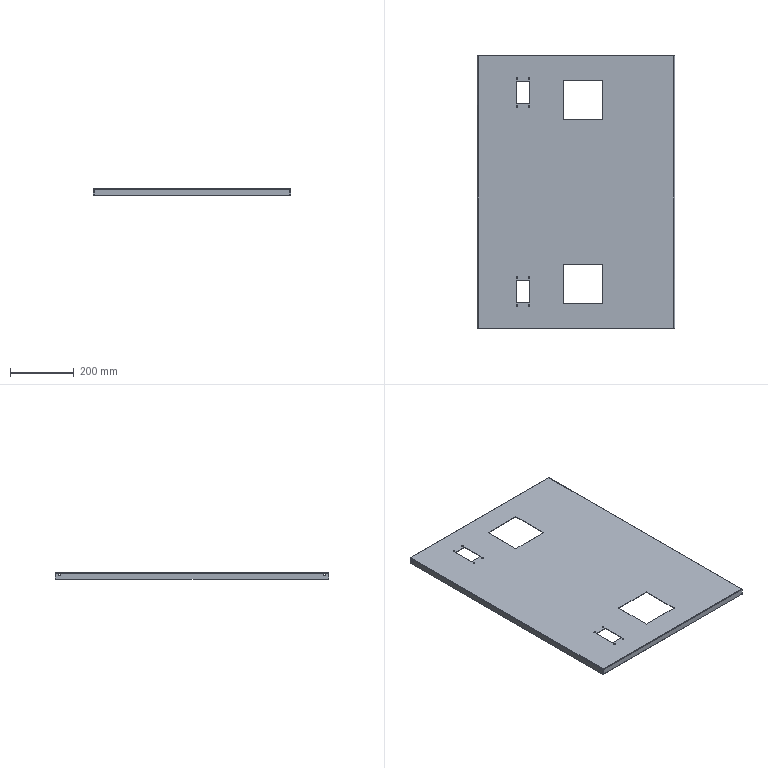Part | STEP file | 001-001-Machine frame end plate | 1 solid | 78 faces | box 618 x 858 x 20 mm | volume 819319 mm3 | plane 38 | cylinder 32 | spline 8 | commonest cylinder face diameters 5 x16 6.5 x8 1.473 x4 4.473 x4